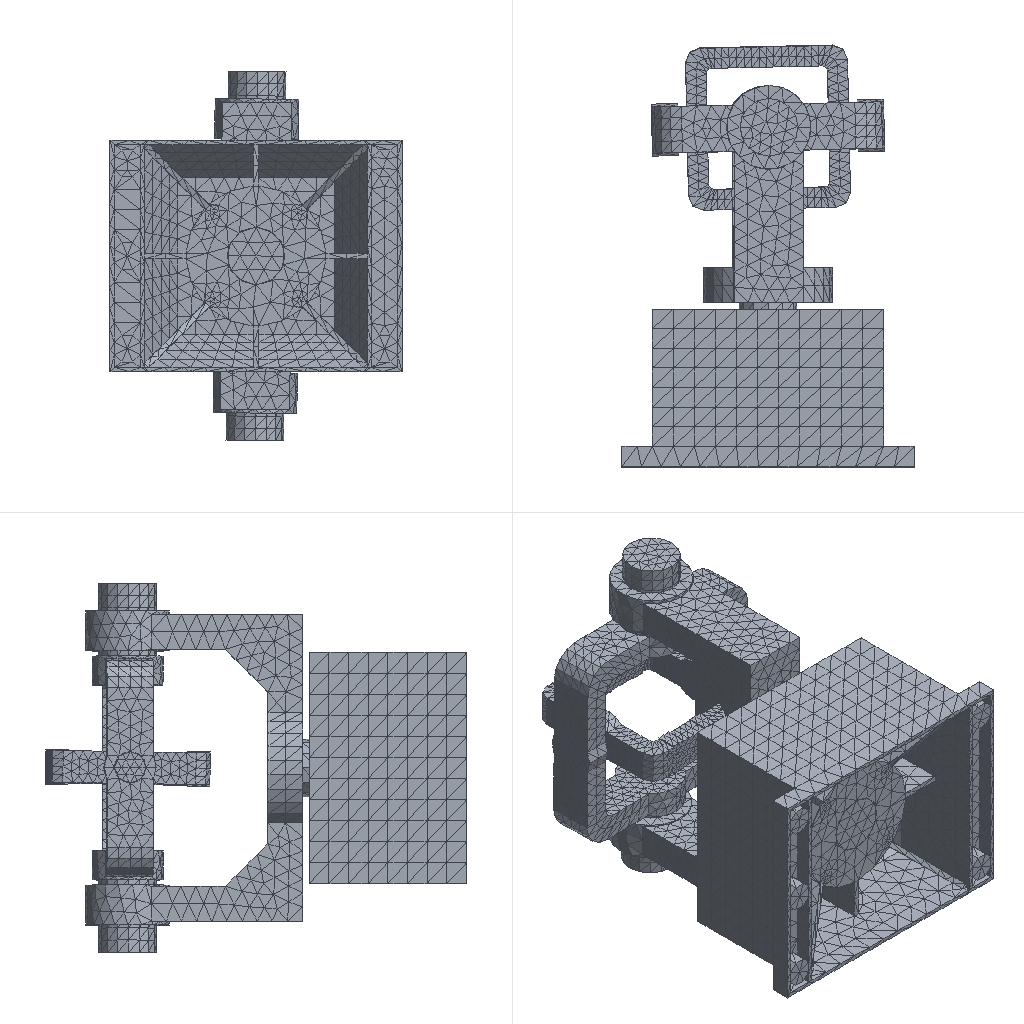Simulation study | abaqus
Set-up summary:
category,name,step,type,value,unit,region
solver,abaqus
solver,version,,,Abaqus/Explicit 2020
units,not stated in the deck,,not stated
analysis,deck,,transient,transient
load_step,Step-1,Step-1,transient
load_step,requested,,,1
mesh,nodes,,,7785
mesh,elements,,,26166
element_type,C3D4,,solid,26166
load,load commands in deck,,count,4
bc,support commands in deck,,count,11
material,MATERIAL-1,,in results
check,setup vs results,,match,"per instance, exact: element labels, types and connectivity; labels of the nodes the elements use; coordinates of those nodes at SINGLE_PRECISION in 4 of 4 instance(s)"
Abaqus input file, long lists of numbers shortened:
*Heading
** Job name: Job-1 Model name: Model-1
** Generated by: Abaqus/CAE 2020
*Preprint, echo=NO, model=NO, history=NO, contact=NO
**
** PARTS
**
*Part, name=sanzhou-1
*Node
      1,  -324.788,   1240.546,   955.672
      2,  -274.801,   1241.635,   955.375
** (1929 more lines like these left out)
*Element, type=C3D4
   1, 1794, 1795, 1796, 1797
   2, 1794, 1798, 1799, 1800
** (6080 more lines like these left out)
*Nset, nset=Set-3, generate
    1,  1931,     1
*Elset, elset=Set-3, generate
    1,  6082,     1
** Section: Section-1
*Solid Section, elset=Set-3, material=Material-1
,
*End Part
**
*Part, name=sanzhou-2
*Node
      1,  -136.781,   1063.571,   1647.002
      2,  -132.423,   863.619,   1646.976
** (2135 more lines like these left out)
*Element, type=C3D4
   1, 1140, 1796, 1125, 1797
   2, 1798, 1799,  839, 1800
** (7397 more lines like these left out)
*Nset, nset=Set-3, generate
    1,  2137,     1
*Elset, elset=Set-3, generate
    1,  7399,     1
** Section: Section-1
*Solid Section, elset=Set-3, material=Material-1
,
*End Part
**
*Part, name=sanzhou-3
*Node
      1,  -40.789,   963.595,   604.414
      2,  -240.786,   963.595,   605.601
** (1573 more lines like these left out)
*Element, type=C3D4
   1, 1291, 1292, 1293, 1294
   2, 1291, 1295, 1296, 1297
** (5545 more lines like these left out)
*Nset, nset=Set-3, generate
    1,  1575,     1
*Elset, elset=Set-3, generate
    1,  5547,     1
** Section: Section-1
*Solid Section, elset=Set-3, material=Material-1
,
*End Part
**
*Part, name=sanzhou-4
*Node
      1,  -538.383,   335.595,        1410.
      2,   261.617,   335.595,        1410.
** (2140 more lines like these left out)
*Element, type=C3D4
   1,  186, 1989,  725, 1208
   2, 1990, 1991, 1992,  363
** (7136 more lines like these left out)
*Nset, nset=Set-3, generate
    1,  2142,     1
*Elset, elset=Set-3, generate
    1,  7138,     1
** Section: Section-1
*Solid Section, elset=Set-3, material=Material-1
,
*End Part
**
**
** ASSEMBLY
**
*Assembly, name=Assembly
**
*Instance, name=sanzhou-1-1, part=sanzhou-1
*End Instance
**
*Instance, name=sanzhou-2-1, part=sanzhou-2
*End Instance
**
*Instance, name=sanzhou-3-1, part=sanzhou-3
*End Instance
**
*Instance, name=sanzhou-4-1, part=sanzhou-4
*End Instance
**
*Node
      1,  -138.383,   963.595,        1010.
*Node
      2,  -138.383,   963.595,        1010.
*Node
      3,  -138.383,   478.595,        1010.
*Nset, nset=Set-1, instance=sanzhou-4-1
  233,  234,  235,  236,  237,  238,  239,  240,  241,  242,  243,  244,  245,  246,  247,  248
  249,  250,  251,  252,  253,  254,  255,  256,  257,  258,  259,  260,  261,  264,  265,  268
** (10 more lines like these left out)
*Elset, elset=Set-1, instance=sanzhou-4-1
 5975, 5978, 5982, 5991, 6004, 6007, 6010, 6011, 6015, 6024, 6026, 6029, 6033, 6042, 6046, 6060
 6062, 6067, 6068, 6076, 6116, 6141, 6143, 6146, 6149, 6152, 6177, 6183, 6185, 6196, 6203, 6211
** (11 more lines like these left out)
*Nset, nset=Set-2, instance=sanzhou-4-1
    1,    2,    3,    4,  156,  157,  158,  159,  261,  262,  263,  264,  265,  266,  267,  268
  285,  286,  287,  288,  289,  290,  291,  292,  293,  294,  295,  296,  297,  298,  299,  300
** (25 more lines like these left out)
*Elset, elset=Set-2, instance=sanzhou-4-1
   80,   82,   83,  100,  131,  148,  175,  212,  233,  242,  264,  267,  280,  282,  285,  288
  303,  315,  324,  325,  335,  341,  425,  426,  435,  445,  461,  474,  514,  587,  589,  642
** (43 more lines like these left out)
*Nset, nset=Set-4
 1,
*Nset, nset=Set-7
 3,
*Nset, nset=Set-8, instance=sanzhou-3-1
   9,  10, 161, 162, 163, 164, 165, 166, 167, 168, 169, 170, 606, 607, 608, 609
 610, 611, 612
*Elset, elset=Set-8, instance=sanzhou-3-1
 1082, 1707, 2436, 2437, 2444, 2455, 2471, 2489, 2496, 2518, 2525, 2543, 2546, 3121, 3260, 3269
 3274, 3314, 3359, 3382, 3518, 3520, 3526, 3588
*Nset, nset=Set-9, instance=sanzhou-3-1
   19,   20,   22,   23,   24,   25,   31,   36,   37,   38,  207,  208,  209,  210,  211,  212
  213,  214,  215,  216,  225,  226,  227,  228,  229,  230,  240,  241,  242,  243,  253,  254
** (9 more lines like these left out)
*Elset, elset=Set-9, instance=sanzhou-3-1
   81,  184,  258,  325,  380,  387,  536,  544,  545,  563,  579,  616,  756,  824,  860,  862
  878,  890,  903,  915,  936,  961,  988, 1076, 1135, 1137, 1199, 1202, 1255, 1320, 1334, 1376
** (15 more lines like these left out)
*Nset, nset=Set-10, instance=sanzhou-2-1
   1,   2,  27,  28, 151, 152, 153, 154, 155, 156, 157, 158, 159, 160, 161, 162
 163, 164, 274, 275, 276, 277, 278, 279, 280, 281, 282, 283, 284, 285, 286, 287
** (2 more lines like these left out)
*Elset, elset=Set-10, instance=sanzhou-2-1
  196,  884,  896,  932, 1000, 1007, 1010, 1312, 1313, 1455, 1459, 1521, 1572, 1896, 2069, 2107
 2527, 2618, 2621, 2682, 2704, 2772, 2866, 2875, 2880, 2889, 2897, 2919, 2922, 2949, 2952, 2970
** (4 more lines like these left out)
*Nset, nset=Set-11, instance=sanzhou-1-1
  41,  42,  47,  48, 257, 258, 259, 260, 261, 262, 263, 264, 265, 266, 269, 270
 271, 272, 273, 274, 275, 276, 277, 278, 801, 802, 803, 804, 805, 806, 807, 808
** (1 more lines like these left out)
*Elset, elset=Set-11, instance=sanzhou-1-1
  167,  249,  331,  776, 1578, 1888, 2511, 2530, 2706, 2720, 2805, 3558, 3573, 3590, 3596, 3609
 3610, 3612, 3625, 3634, 3638, 3648, 3699, 3720, 3749, 3766, 3774, 3782, 3811, 3830, 3979, 3988
** (1 more lines like these left out)
*Nset, nset=m_Set-3
 1,
*Nset, nset=m_Set-5
 2,
*Nset, nset=m_Set-6
 3,
*Elset, elset=_s_Surf-1_S3, internal, instance=sanzhou-1-1
  167,  776, 1578, 1888, 2530, 2720, 2805, 3558, 3573, 3590, 3596, 3609, 3610, 3612, 3625, 3634
 3638, 3648, 3699, 3720, 3749, 3766, 3774, 3782, 3811, 3979, 3988, 4971, 4978, 5070, 5080, 5106
** (1 more lines like these left out)
*Elset, elset=_s_Surf-1_S4, internal, instance=sanzhou-1-1
  249,  331, 3830, 4993
*Elset, elset=_s_Surf-1_S2, internal, instance=sanzhou-1-1
 2511, 2706, 5024, 5761, 5876
*Surface, type=ELEMENT, name=s_Surf-1
_s_Surf-1_S3, S3
_s_Surf-1_S4, S4
_s_Surf-1_S2, S2
*Elset, elset=_s_Surf-2_S3, internal, instance=sanzhou-2-1
  196,  884,  896,  932, 1000, 1007, 1010, 1312, 1313, 1459, 1521, 1572, 2069, 2107, 2527, 2618
 2621, 2682, 2704, 2772, 2866, 2875, 2880, 2889, 2897, 2919, 2922, 2949, 2970, 2978, 3053, 3072
** (3 more lines like these left out)
*Elset, elset=_s_Surf-2_S4, internal, instance=sanzhou-2-1
 1455, 2952
*Elset, elset=_s_Surf-2_S1, internal, instance=sanzhou-2-1
 1896, 3448, 6396, 6811
*Elset, elset=_s_Surf-2_S2, internal, instance=sanzhou-2-1
 6959,
*Surface, type=ELEMENT, name=s_Surf-2
_s_Surf-2_S3, S3
_s_Surf-2_S4, S4
_s_Surf-2_S2, S2
_s_Surf-2_S1, S1
*Elset, elset=_s_Surf-3_S3, internal, instance=sanzhou-3-1
  116,  293,  332,  354,  392,  425,  426,  491,  523,  543,  564,  573,  630,  690,  705,  716
  797,  798,  829,  866,  867,  871,  875,  878,  931,  937,  954,  970,  972, 1055, 1072, 1073
** (25 more lines like these left out)
*Elset, elset=_s_Surf-3_S4, internal, instance=sanzhou-3-1
  139,  450,  466,  538,  674,  725,  727, 1065, 1536, 1836, 1870, 1931, 1979, 2005, 2015, 2051
 2183, 2187, 2191, 2235, 2260, 2380, 2424, 2620, 2634, 2640, 2645, 2670, 2681, 2698, 2716, 2723
** (6 more lines like these left out)
*Elset, elset=_s_Surf-3_S1, internal, instance=sanzhou-3-1
  445, 2039, 2045, 2093, 2112, 2199, 2210, 2258, 2307, 2324, 2335, 2345, 2400, 2569, 2592, 2625
 2627, 2653, 2659, 2662, 2676, 2726, 2745, 2752, 2829, 2834, 2883, 3037, 3054, 3377, 3402, 3739
** (3 more lines like these left out)
*Elset, elset=_s_Surf-3_S2, internal, instance=sanzhou-3-1
   47,   97,  435,  541,  593, 1160, 1465, 1743, 1833, 1930, 2033, 2067, 2310, 2370, 2407, 2409
 2603, 2614, 2617, 2641, 2657, 2684, 2706, 2722, 2741, 2765, 2790, 2870, 2892, 2914, 2963, 3027
** (4 more lines like these left out)
*Surface, type=ELEMENT, name=s_Surf-3
_s_Surf-3_S3, S3
_s_Surf-3_S4, S4
_s_Surf-3_S2, S2
_s_Surf-3_S1, S1
*Elset, elset=_s_Surf-4_S2, internal, instance=sanzhou-1-1
    3, 1141, 1210, 1270, 1286, 1322, 1336, 1346, 1358, 1394, 1432, 1455, 1485, 1514, 1564, 1628
 1906, 1972, 1988, 2024, 2033, 2046, 2052, 2066, 2168, 2216, 2227, 2264, 2566, 2618, 2698, 2776
** (5 more lines like these left out)
*Elset, elset=_s_Surf-4_S3, internal, instance=sanzhou-1-1
   35,   50,   73,   78,  126,  239,  283,  311,  376,  482,  530,  538,  547,  713,  761,  987
  989, 1107, 1148, 1253, 1288, 1294, 1295, 1301, 1310, 1314, 1315, 1320, 1326, 1337, 1339, 1373
** (25 more lines like these left out)
*Elset, elset=_s_Surf-4_S1, internal, instance=sanzhou-1-1
 1039, 1221, 1296, 1304, 1316, 1327, 1335, 1342, 1362, 1422, 1425, 1495, 1529, 1561, 1600, 2035
 2038, 2631, 2658, 2754, 2755, 2772, 2773, 2777, 2810, 2841, 2877, 2969, 3004, 3023, 3067, 3189
** (2 more lines like these left out)
*Elset, elset=_s_Surf-4_S4, internal, instance=sanzhou-1-1
  567, 1140, 1177, 1267, 1290, 1293, 1309, 1347, 1349, 1351, 1483, 1490, 1499, 1540, 1586, 1681
 1697, 1929, 1970, 1989, 2005, 2015, 2044, 2047, 2051, 2121, 2162, 2191, 2562, 2581, 2611, 2665
** (7 more lines like these left out)
*Surface, type=ELEMENT, name=s_Surf-4
_s_Surf-4_S2, S2
_s_Surf-4_S3, S3
_s_Surf-4_S4, S4
_s_Surf-4_S1, S1
*Elset, elset=_s_Surf-5_S2, internal, instance=sanzhou-2-1
  136,  175,  517,  525, 1539, 1806, 1881, 2077, 2086, 2088, 2099, 2162, 2194, 2337, 2394, 2416
 2419, 2438, 2467, 2655, 2661, 2720, 2778, 2836, 3003, 3160, 3219, 3452, 3460, 3502, 3576, 3628
** (7 more lines like these left out)
*Elset, elset=_s_Surf-5_S1, internal, instance=sanzhou-2-1
  854, 1039, 1151, 1622, 1916, 1988, 2078, 2141, 2142, 2144, 2242, 2290, 2296, 2376, 2448, 2461
 2515, 2528, 2538, 2715, 2794, 2988, 3095, 3155, 3207, 3490, 3563, 3579, 3597, 3625, 3626, 3649
** (5 more lines like these left out)
*Elset, elset=_s_Surf-5_S3, internal, instance=sanzhou-2-1
  550,  554,  649,  849,  918,  938, 1052, 1053, 1060, 1094, 1125, 1129, 1222, 1333, 1538, 1586
 1658, 1676, 1696, 1736, 1743, 1748, 1759, 1831, 1841, 1882, 1884, 1913, 1918, 1982, 2034, 2038
** (15 more lines like these left out)
*Elset, elset=_s_Surf-5_S4, internal, instance=sanzhou-2-1
  114,  130,  186,  191,  304,  403,  557,  702,  729, 1407, 2082, 2093, 2133, 2178, 2189, 2238
 2295, 2338, 2503, 2537, 2651, 2681, 2766, 3027, 3031, 3037, 3054, 3089, 3098, 3131, 3266, 3306
** (6 more lines like these left out)
*Surface, type=ELEMENT, name=s_Surf-5
_s_Surf-5_S2, S2
_s_Surf-5_S1, S1
_s_Surf-5_S4, S4
_s_Surf-5_S3, S3
*Elset, elset=_s_Surf-6_S2, internal, instance=sanzhou-2-1
   66,   73,  136,  175,  517,  525,  804, 1539, 1806, 1881, 1902, 2077, 2086, 2088, 2099, 2111
 2162, 2194, 2337, 2394, 2416, 2419, 2438, 2467, 2618, 2655, 2661, 2720, 2778, 2836, 2927, 3003
** (8 more lines like these left out)
*Elset, elset=_s_Surf-6_S1, internal, instance=sanzhou-2-1
  854, 1039, 1151, 1183, 1622, 1715, 1909, 1916, 1988, 2078, 2141, 2142, 2144, 2242, 2290, 2296
 2376, 2448, 2461, 2515, 2528, 2538, 2682, 2715, 2794, 2902, 2988, 3095, 3155, 3207, 3490, 3563
** (6 more lines like these left out)
*Elset, elset=_s_Surf-6_S3, internal, instance=sanzhou-2-1
  138,  550,  554,  603,  639,  649,  677,  723,  782,  849,  885,  895,  900,  902,  906,  918
  926,  938,  999, 1006, 1052, 1053, 1060, 1094, 1125, 1129, 1194, 1199, 1222, 1271, 1273, 1274
** (35 more lines like these left out)
*Elset, elset=_s_Surf-6_S4, internal, instance=sanzhou-2-1
  114,  130,  186,  191,  228,  304,  403,  484,  557,  702,  729,  908, 1184, 1295, 1407, 1636
 1656, 1896, 1908, 1937, 2082, 2093, 2133, 2178, 2189, 2238, 2295, 2338, 2503, 2537, 2651, 2681
** (7 more lines like these left out)
*Surface, type=ELEMENT, name=s_Surf-6
_s_Surf-6_S2, S2
_s_Surf-6_S1, S1
_s_Surf-6_S4, S4
_s_Surf-6_S3, S3
*Elset, elset=_s_Surf-7_S2, internal, instance=sanzhou-1-1
    3,  249, 1141, 1210, 1270, 1286, 1322, 1336, 1346, 1358, 1394, 1432, 1455, 1485, 1514, 1564
 1628, 1906, 1972, 1988, 2024, 2033, 2046, 2052, 2066, 2168, 2212, 2216, 2227, 2264, 2566, 2618
** (6 more lines like these left out)
*Elset, elset=_s_Surf-7_S3, internal, instance=sanzhou-1-1
   35,   42,   50,   73,   78,   80,  126,  185,  239,  283,  311,  316,  376,  446,  448,  449
  464,  482,  493,  494,  508,  530,  538,  547,  620,  622,  640,  642,  683,  701,  713,  761
** (34 more lines like these left out)
*Elset, elset=_s_Surf-7_S1, internal, instance=sanzhou-1-1
  166, 1032, 1039, 1221, 1296, 1304, 1316, 1327, 1335, 1342, 1362, 1422, 1425, 1495, 1529, 1561
 1600, 2035, 2038, 2631, 2658, 2754, 2755, 2772, 2773, 2777, 2783, 2810, 2841, 2877, 2888, 2969
** (3 more lines like these left out)
*Elset, elset=_s_Surf-7_S4, internal, instance=sanzhou-1-1
  181,  315,  505,  539,  567,  598,  977, 1140, 1177, 1267, 1290, 1293, 1309, 1347, 1349, 1351
 1442, 1483, 1490, 1499, 1540, 1586, 1681, 1697, 1929, 1970, 1989, 2005, 2015, 2044, 2047, 2051
** (8 more lines like these left out)
*Surface, type=ELEMENT, name=s_Surf-7
_s_Surf-7_S2, S2
_s_Surf-7_S3, S3
_s_Surf-7_S4, S4
_s_Surf-7_S1, S1
** Constraint: Constraint-1
*Coupling, constraint name=Constraint-1, ref node=m_Set-3, surface=s_Surf-7
*Kinematic
** Constraint: Constraint-2
*Coupling, constraint name=Constraint-2, ref node=m_Set-5, surface=s_Surf-6
*Kinematic
** Constraint: Constraint-3
*Coupling, constraint name=Constraint-3, ref node=m_Set-6, surface=s_Surf-3
*Kinematic
*End Assembly
**
** MATERIALS
**
*Material, name=Material-1
*Density
 7.8e-09,
*Elastic
206000., 0.3
**
** INTERACTION PROPERTIES
**
*Surface Interaction, name=IntProp-1
*Friction
 0.02,
*Surface Behavior, pressure-overclosure=HARD
** ----------------------------------------------------------------
**
** STEP: Step-1
**
*Step, name=Step-1, nlgeom=YES
*Dynamic, Explicit
, 0.1
*Bulk Viscosity
0.06, 1.2
**
** BOUNDARY CONDITIONS
**
** Name: BC-1 Type: 对称/反对称/完全固定
*Boundary
Set-2, ENCASTRE
** Name: BC-2 Type: 速度/角速度
*Boundary, type=VELOCITY
Set-4, 4, 4, 62.8
** Name: BC-3 Type: 速度/角速度
*Boundary, type=VELOCITY
m_Set-5, 6, 6, 50.24
** Name: BC-4 Type: 速度/角速度
*Boundary, type=VELOCITY
Set-7, 5, 5, 37.68
** Name: BC-5 Type: 位移/转角
*Boundary
Set-9, 2, 2
Set-9, 4, 4
Set-9, 6, 6
** Name: BC-6 Type: 位移/转角
*Boundary
Set-10, 4, 4
Set-10, 5, 5
** Name: BC-7 Type: 位移/转角
*Boundary
Set-11, 5, 5
Set-11, 6, 6
**
** LOADS
**
** Name: Load-1   Type: Gravity
*Dload
, GRAV, 9800., 0., -1., 0.
**
** INTERACTIONS
**
** Interaction: Int-1
*Contact, op=NEW
*Contact Inclusions, ALL EXTERIOR
*Contact Property Assignment
 ,  , IntProp-1
**
** OUTPUT REQUESTS
**
*Restart, write, number interval=1, time marks=NO
**
** FIELD OUTPUT: F-Output-1
**
*Output, field, number interval=100
*Node Output
A, AR, AT, CF, RF, RM, RT, U
UR, UT, V, VR, VT
*Element Output, directions=YES
E, EVF, LE, MISES, MISESMAX, MISESONLY, PE, PEEQ, PEEQMAX, PEEQT, PEEQVAVG, PEMAG, PEVAVG, S, SF, SSAVG
SVAVG, VE, YIELDPOT
*Contact Output
CDISP, CSTRESS
**
** HISTORY OUTPUT: H-Output-1
**
*Output, history, variable=PRESELECT
*End Step
Results summary:
result,step,Step-1,partial,increments=87928 time=0.04/0.1
result,analysis,,,transient
result,last_loadstep,,,1
result,primary field,,,U
result,reaction total,,FX,8136887.992,model units
result,reaction total,,FY,27133561.809,model units
result,reaction total,,FZ,13159584.919,model units